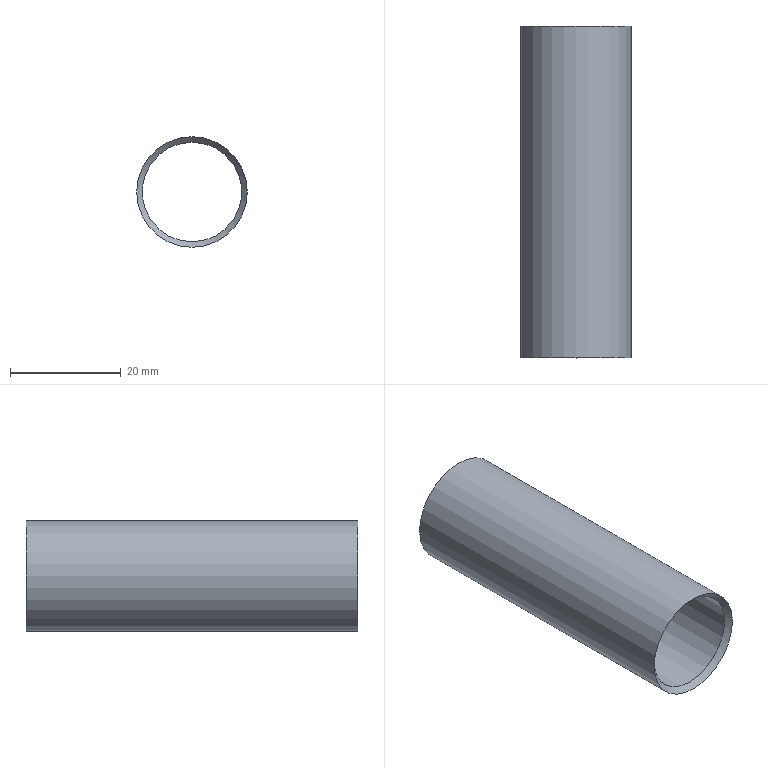Part | STEP file | JBJ-P-1010-02 | 1 solid | 4 faces | box 20 x 60 x 20 mm | volume 3552 mm3 | cylinder 2 | plane 1 | cone 1 | commonest cylinder face diameters 18 x1 20 x1
STEP:
#1=CARTESIAN_POINT('',(0.,60.,10.));
#2=VERTEX_POINT('',#1);
#3=CARTESIAN_POINT('',(0.,60.,0.));
#4=DIRECTION('',(0.,1.,0.));
#5=DIRECTION('',(0.,0.,1.));
#6=AXIS2_PLACEMENT_3D('',#3,#4,#5);
#7=CIRCLE('',#6,10.);
#8=EDGE_CURVE('',#2,#2,#7,.T.);
#9=ORIENTED_EDGE('',*,*,#8,.T.);
#10=EDGE_LOOP('',(#9));
#11=FACE_OUTER_BOUND('',#10,.T.);
#12=CARTESIAN_POINT('',(0.,60.,9.));
#13=VERTEX_POINT('',#12);
#14=CARTESIAN_POINT('',(0.,60.,0.));
#15=DIRECTION('',(0.,1.,0.));
#16=DIRECTION('',(0.,0.,1.));
#17=AXIS2_PLACEMENT_3D('',#14,#15,#16);
#18=CIRCLE('',#17,9.);
#19=EDGE_CURVE('',#13,#13,#18,.T.);
#20=ORIENTED_EDGE('',*,*,#19,.F.);
#21=EDGE_LOOP('',(#20));
#22=FACE_BOUND('',#21,.T.);
#23=CARTESIAN_POINT('',(0.,60.,0.));
#24=DIRECTION('',(0.,1.,0.));
#25=DIRECTION('',(0.,0.,1.));
#26=AXIS2_PLACEMENT_3D('',#23,#24,#25);
#27=PLANE('',#26);
#28=ADVANCED_FACE('',(#11,#22),#27,.T.);
#29=ORIENTED_EDGE('',*,*,#8,.F.);
#30=EDGE_LOOP('',(#29));
#31=FACE_OUTER_BOUND('',#30,.T.);
#32=CARTESIAN_POINT('',(0.,0.,10.));
#33=VERTEX_POINT('',#32);
#34=CARTESIAN_POINT('',(0.,0.,0.));
#35=DIRECTION('',(0.,1.,0.));
#36=DIRECTION('',(0.,0.,1.));
#37=AXIS2_PLACEMENT_3D('',#34,#35,#36);
#38=CIRCLE('',#37,10.);
#39=EDGE_CURVE('',#33,#33,#38,.T.);
#40=ORIENTED_EDGE('',*,*,#39,.T.);
#41=EDGE_LOOP('',(#40));
#42=FACE_OUTER_BOUND('',#41,.T.);
#43=CARTESIAN_POINT('',(0.,60.,0.));
#44=DIRECTION('',(0.,-1.,0.));
#45=DIRECTION('',(0.,0.,-1.));
#46=AXIS2_PLACEMENT_3D('',#43,#44,#45);
#47=CYLINDRICAL_SURFACE('',#46,10.);
#48=ADVANCED_FACE('',(#31,#42),#47,.T.);
#49=CARTESIAN_POINT('',(0.,1.,9.));
#50=VERTEX_POINT('',#49);
#51=CARTESIAN_POINT('',(0.,1.,0.));
#52=DIRECTION('',(0.,-1.,0.));
#53=DIRECTION('',(0.,0.,1.));
#54=AXIS2_PLACEMENT_3D('',#51,#52,#53);
#55=CIRCLE('',#54,9.);
#56=EDGE_CURVE('',#50,#50,#55,.T.);
#57=ORIENTED_EDGE('',*,*,#56,.T.);
#58=EDGE_LOOP('',(#57));
#59=FACE_OUTER_BOUND('',#58,.T.);
#60=ORIENTED_EDGE('',*,*,#19,.T.);
#61=EDGE_LOOP('',(#60));
#62=FACE_OUTER_BOUND('',#61,.T.);
#63=CARTESIAN_POINT('',(0.,60.,0.));
#64=DIRECTION('',(0.,-1.,0.));
#65=DIRECTION('',(0.,0.,-1.));
#66=AXIS2_PLACEMENT_3D('',#63,#64,#65);
#67=CYLINDRICAL_SURFACE('',#66,9.);
#68=ADVANCED_FACE('',(#59,#62),#67,.F.);
#69=ORIENTED_EDGE('',*,*,#56,.F.);
#70=EDGE_LOOP('',(#69));
#71=FACE_BOUND('',#70,.T.);
#72=ORIENTED_EDGE('',*,*,#39,.F.);
#73=EDGE_LOOP('',(#72));
#74=FACE_OUTER_BOUND('',#73,.T.);
#75=CARTESIAN_POINT('',(0.,0.,0.));
#76=DIRECTION('',(0.,-1.,0.));
#77=DIRECTION('',(0.,0.,-1.));
#78=AXIS2_PLACEMENT_3D('',#75,#76,#77);
#79=CONICAL_SURFACE('',#78,10.,0.7854);
#80=ADVANCED_FACE('',(#71,#74),#79,.F.);
#81=CLOSED_SHELL('',(#28,#48,#68,#80));
#82=MANIFOLD_SOLID_BREP('',#81);
#83=CARTESIAN_POINT('',(0.,0.,0.));
#84=DIRECTION('',(0.,0.,1.));
#85=DIRECTION('',(1.,0.,0.));
#86=AXIS2_PLACEMENT_3D('',#83,#84,#85);
#87=(LENGTH_UNIT()NAMED_UNIT(*)SI_UNIT(.MILLI.,.METRE.));
#88=UNCERTAINTY_MEASURE_WITH_UNIT(LENGTH_MEASURE(0.00001),#87,'','');
#89=(NAMED_UNIT(*)PLANE_ANGLE_UNIT()SI_UNIT($,.RADIAN.));
#90=(NAMED_UNIT(*)SI_UNIT($,.STERADIAN.)SOLID_ANGLE_UNIT());
#91=(GEOMETRIC_REPRESENTATION_CONTEXT(3)GLOBAL_UNCERTAINTY_ASSIGNED_CONTEXT((#88))GLOBAL_UNIT_ASSIGNED_CONTEXT((#87,#89,#90))REPRESENTATION_CONTEXT('',''));
#92=ADVANCED_BREP_SHAPE_REPRESENTATION('',(#82,#86),#91);